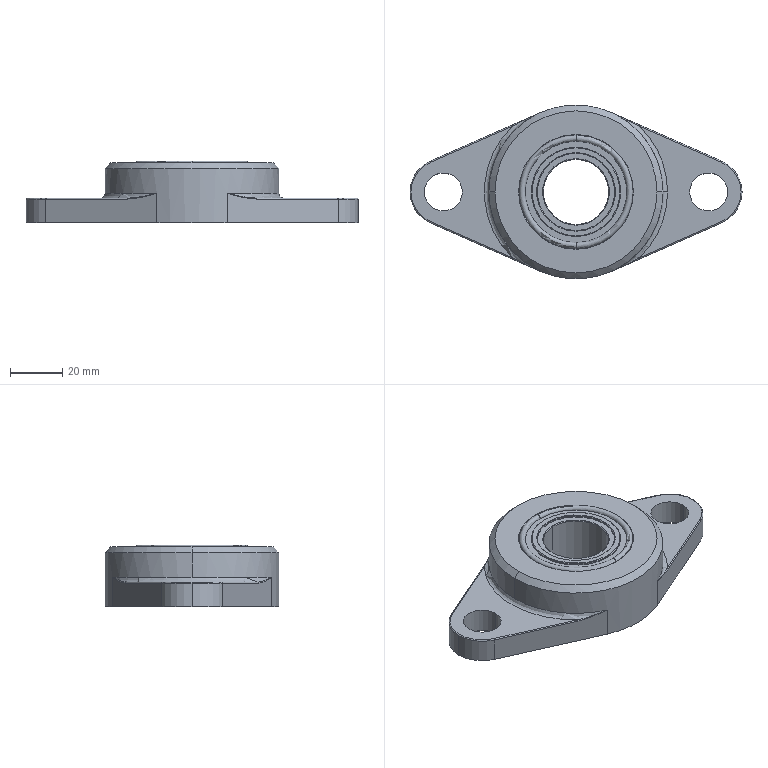Part | SolidWorks | features BaseBody 2 | 2 solids | 74 faces | box 127 x 66.5 x 23.653 mm | volume 83435 mm3 | cylinder 29 | cone 18 | plane 15 | torus 8 | spline 4 | commonest cylinder face diameters 0.762 x4 14.5 x4 29.593 x4 34.207 x4 43.433 x4 25.5 x3